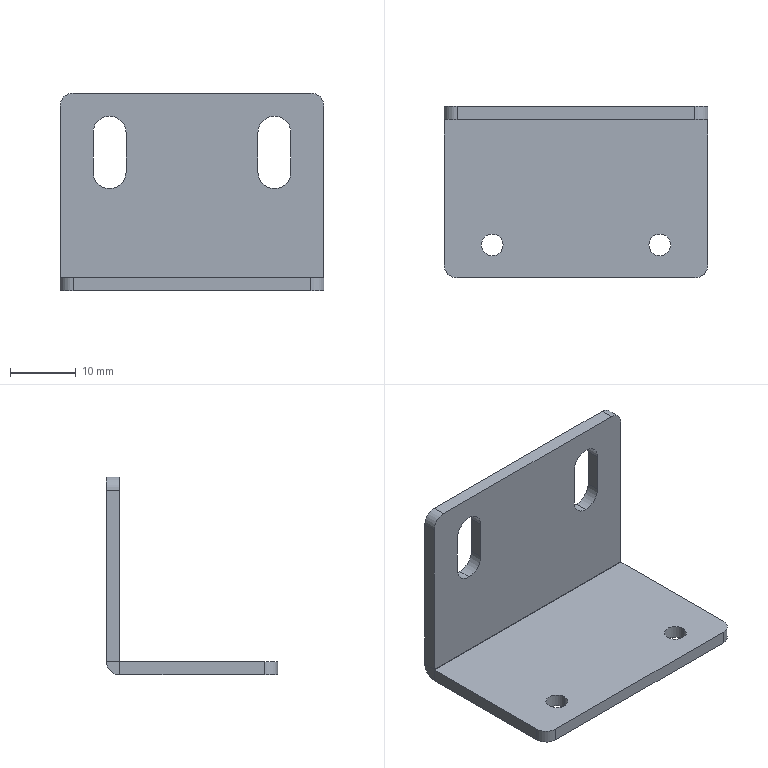Part | STEP file | Limit switch fixing plate 2 | 1 solid | 32 faces | box 40 x 26 x 30 mm | volume 4044 mm3 | cylinder 16 | plane 16 | commonest cylinder face diameters 5 x6 3.3 x4 4 x4 0.1 x1 4.1 x1